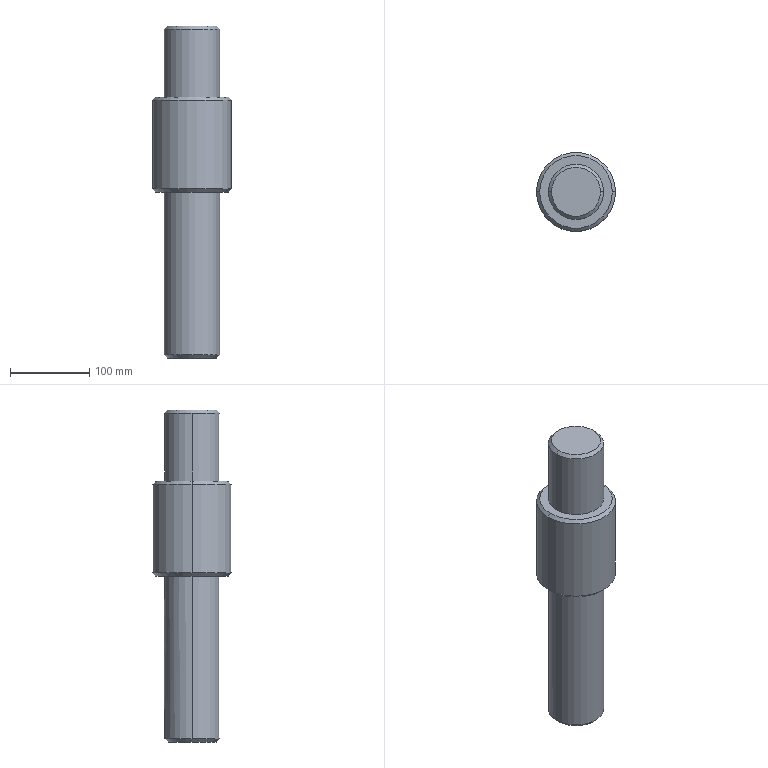Part | SolidWorks | features ICE 2, Chamfer 1, Extrusion 1 | 1 solid | 24 faces | box 100 x 100 x 420 mm | volume 2082883 mm3 | cone 9 | cylinder 8 | plane 7 | commonest cylinder face diameters 70 x4 15 x2 100 x2
STEP:
#1=CARTESIAN_POINT('',(0.,25.,-227.5));
#2=VERTEX_POINT('',#1);
#3=CARTESIAN_POINT('',(7.5,25.,-235.));
#4=VERTEX_POINT('',#3);
#5=CARTESIAN_POINT('',(0.,25.,-235.));
#6=DIRECTION('',(0.,1.,0.));
#7=DIRECTION('',(0.,0.,1.));
#8=AXIS2_PLACEMENT_3D('',#5,#6,#7);
#9=CIRCLE('',#8,7.5);
#10=EDGE_CURVE('',#2,#4,#9,.T.);
#11=ORIENTED_EDGE('',*,*,#10,.F.);
#12=CARTESIAN_POINT('',(0.,35.,-227.5));
#13=VERTEX_POINT('',#12);
#14=CARTESIAN_POINT('',(0.,25.,-227.5));
#15=DIRECTION('',(0.,1.,0.));
#16=VECTOR('',#15,1000.);
#17=LINE('',#14,#16);
#18=EDGE_CURVE('',#2,#13,#17,.T.);
#19=ORIENTED_EDGE('',*,*,#18,.T.);
#20=CARTESIAN_POINT('',(7.5,34.187,-235.));
#21=VERTEX_POINT('',#20);
#22=CARTESIAN_POINT('',(0.,35.,-227.5));
#23=CARTESIAN_POINT('',(0.4904,35.,-227.5));
#24=CARTESIAN_POINT('',(0.9887,34.989,-227.549));
#25=CARTESIAN_POINT('',(1.951,34.949,-227.742));
#26=CARTESIAN_POINT('',(2.419,34.919,-227.884));
#27=CARTESIAN_POINT('',(3.101,34.863,-228.167));
#28=CARTESIAN_POINT('',(3.325,34.842,-228.273));
#29=CARTESIAN_POINT('',(3.758,34.798,-228.505));
#30=CARTESIAN_POINT('',(3.967,34.775,-228.63));
#31=CARTESIAN_POINT('',(4.372,34.726,-228.901));
#32=CARTESIAN_POINT('',(4.568,34.701,-229.047));
#33=CARTESIAN_POINT('',(4.946,34.649,-229.357));
#34=CARTESIAN_POINT('',(5.129,34.623,-229.522));
#35=CARTESIAN_POINT('',(5.651,34.543,-230.044));
#36=CARTESIAN_POINT('',(5.96,34.49,-230.421));
#37=CARTESIAN_POINT('',(6.367,34.416,-231.029));
#38=CARTESIAN_POINT('',(6.493,34.393,-231.238));
#39=CARTESIAN_POINT('',(6.726,34.348,-231.673));
#40=CARTESIAN_POINT('',(6.832,34.327,-231.896));
#41=CARTESIAN_POINT('',(7.114,34.27,-232.575));
#42=CARTESIAN_POINT('',(7.257,34.24,-233.043));
#43=CARTESIAN_POINT('',(7.45,34.198,-234.006));
#44=CARTESIAN_POINT('',(7.5,34.187,-234.503));
#45=CARTESIAN_POINT('',(7.5,34.187,-235.));
#46=B_SPLINE_CURVE_WITH_KNOTS('',3,(#22,#23,#24,#25,#26,#27,#28,#29,#30,#31,#32,#33,#34,#35,#36,#37,#38,#39,#40,#41,#42,#43,#44,#45),.UNSPECIFIED.,.F.,.F.,(4,2,2,2,2,2,2,2,2,2,2,4),(0.01176,0.01323,0.0147,0.01543,0.01617,0.0169,0.01764,0.0191,0.01984,0.02057,0.02204,0.02351),.UNSPECIFIED.);
#47=EDGE_CURVE('',#13,#21,#46,.T.);
#48=ORIENTED_EDGE('',*,*,#47,.T.);
#49=CARTESIAN_POINT('',(7.5,25.,-235.));
#50=DIRECTION('',(0.,1.,0.));
#51=VECTOR('',#50,1000.);
#52=LINE('',#49,#51);
#53=EDGE_CURVE('',#4,#21,#52,.T.);
#54=ORIENTED_EDGE('',*,*,#53,.F.);
#55=EDGE_LOOP('',(#11,#19,#48,#54));
#56=FACE_OUTER_BOUND('',#55,.T.);
#57=CARTESIAN_POINT('',(0.,25.,-235.));
#58=DIRECTION('',(0.,1.,0.));
#59=DIRECTION('',(0.,0.,1.));
#60=AXIS2_PLACEMENT_3D('',#57,#58,#59);
#61=CYLINDRICAL_SURFACE('',#60,7.5);
#62=ADVANCED_FACE('',(#56),#61,.F.);
#63=CARTESIAN_POINT('',(-31.,0.,-270.));
#64=VERTEX_POINT('',#63);
#65=CARTESIAN_POINT('',(-7.5,30.079,-270.));
#66=VERTEX_POINT('',#65);
#67=CARTESIAN_POINT('',(0.,0.,-270.));
#68=DIRECTION('',(0.,0.,-1.));
#69=DIRECTION('',(1.,0.,0.));
#70=AXIS2_PLACEMENT_3D('',#67,#68,#69);
#71=CIRCLE('',#70,31.);
#72=EDGE_CURVE('',#64,#66,#71,.T.);
#73=ORIENTED_EDGE('',*,*,#72,.F.);
#74=CARTESIAN_POINT('',(-35.,0.,-266.));
#75=VERTEX_POINT('',#74);
#76=CARTESIAN_POINT('',(-35.,0.,-266.));
#77=DIRECTION('',(-0.7071,0.,0.7071));
#78=VECTOR('',#77,1000.);
#79=LINE('',#76,#78);
#80=EDGE_CURVE('',#64,#75,#79,.T.);
#81=ORIENTED_EDGE('',*,*,#80,.T.);
#82=CARTESIAN_POINT('',(-7.5,34.187,-266.));
#83=VERTEX_POINT('',#82);
#84=CARTESIAN_POINT('',(0.,0.,-266.));
#85=DIRECTION('',(0.,0.,1.));
#86=DIRECTION('',(1.,0.,0.));
#87=AXIS2_PLACEMENT_3D('',#84,#85,#86);
#88=CIRCLE('',#87,35.);
#89=EDGE_CURVE('',#83,#75,#88,.T.);
#90=ORIENTED_EDGE('',*,*,#89,.F.);
#91=CARTESIAN_POINT('',(-7.5,30.079,-270.));
#92=CARTESIAN_POINT('',(-7.5,31.451,-268.669));
#93=CARTESIAN_POINT('',(-7.5,32.82,-267.335));
#94=CARTESIAN_POINT('',(-7.5,34.187,-266.));
#95=B_SPLINE_CURVE_WITH_KNOTS('',3,(#91,#92,#93,#94),.UNSPECIFIED.,.F.,.F.,(4,4),(0.0194,0.02513),.UNSPECIFIED.);
#96=EDGE_CURVE('',#66,#83,#95,.T.);
#97=ORIENTED_EDGE('',*,*,#96,.F.);
#98=EDGE_LOOP('',(#73,#81,#90,#97));
#99=FACE_OUTER_BOUND('',#98,.T.);
#100=CARTESIAN_POINT('',(0.,0.,-266.));
#101=DIRECTION('',(0.,0.,1.));
#102=DIRECTION('',(1.,0.,0.));
#103=AXIS2_PLACEMENT_3D('',#100,#101,#102);
#104=CONICAL_SURFACE('',#103,35.,0.7854);
#105=ADVANCED_FACE('',(#99),#104,.T.);
#106=ORIENTED_EDGE('',*,*,#80,.F.);
#107=CARTESIAN_POINT('',(31.,0.,-270.));
#108=VERTEX_POINT('',#107);
#109=CARTESIAN_POINT('',(0.,0.,-270.));
#110=DIRECTION('',(0.,0.,-1.));
#111=DIRECTION('',(1.,0.,0.));
#112=AXIS2_PLACEMENT_3D('',#109,#110,#111);
#113=CIRCLE('',#112,31.);
#114=EDGE_CURVE('',#108,#64,#113,.T.);
#115=ORIENTED_EDGE('',*,*,#114,.F.);
#116=CARTESIAN_POINT('',(35.,0.,-266.));
#117=VERTEX_POINT('',#116);
#118=CARTESIAN_POINT('',(35.,0.,-266.));
#119=DIRECTION('',(0.7071,0.,0.7071));
#120=VECTOR('',#119,1000.);
#121=LINE('',#118,#120);
#122=EDGE_CURVE('',#108,#117,#121,.T.);
#123=ORIENTED_EDGE('',*,*,#122,.T.);
#124=CARTESIAN_POINT('',(0.,0.,-266.));
#125=DIRECTION('',(0.,0.,1.));
#126=DIRECTION('',(1.,0.,0.));
#127=AXIS2_PLACEMENT_3D('',#124,#125,#126);
#128=CIRCLE('',#127,35.);
#129=EDGE_CURVE('',#75,#117,#128,.T.);
#130=ORIENTED_EDGE('',*,*,#129,.F.);
#131=EDGE_LOOP('',(#106,#115,#123,#130));
#132=FACE_OUTER_BOUND('',#131,.T.);
#133=CARTESIAN_POINT('',(0.,0.,-266.));
#134=DIRECTION('',(0.,0.,1.));
#135=DIRECTION('',(1.,0.,0.));
#136=AXIS2_PLACEMENT_3D('',#133,#134,#135);
#137=CONICAL_SURFACE('',#136,35.,0.7854);
#138=ADVANCED_FACE('',(#132),#137,.T.);
#139=CARTESIAN_POINT('',(31.,0.,150.));
#140=VERTEX_POINT('',#139);
#141=CARTESIAN_POINT('',(-31.,0.,150.));
#142=VERTEX_POINT('',#141);
#143=CARTESIAN_POINT('',(0.,0.,150.));
#144=DIRECTION('',(0.,0.,1.));
#145=DIRECTION('',(1.,0.,0.));
#146=AXIS2_PLACEMENT_3D('',#143,#144,#145);
#147=CIRCLE('',#146,31.);
#148=EDGE_CURVE('',#140,#142,#147,.T.);
#149=ORIENTED_EDGE('',*,*,#148,.F.);
#150=CARTESIAN_POINT('',(35.,0.,146.));
#151=VERTEX_POINT('',#150);
#152=CARTESIAN_POINT('',(31.,0.,150.));
#153=DIRECTION('',(0.7071,0.,-0.7071));
#154=VECTOR('',#153,1000.);
#155=LINE('',#152,#154);
#156=EDGE_CURVE('',#140,#151,#155,.T.);
#157=ORIENTED_EDGE('',*,*,#156,.T.);
#158=CARTESIAN_POINT('',(-35.,0.,146.));
#159=VERTEX_POINT('',#158);
#160=CARTESIAN_POINT('',(0.,0.,146.));
#161=DIRECTION('',(0.,0.,-1.));
#162=DIRECTION('',(1.,0.,0.));
#163=AXIS2_PLACEMENT_3D('',#160,#161,#162);
#164=CIRCLE('',#163,35.);
#165=EDGE_CURVE('',#159,#151,#164,.T.);
#166=ORIENTED_EDGE('',*,*,#165,.F.);
#167=CARTESIAN_POINT('',(-31.,0.,150.));
#168=DIRECTION('',(-0.7071,0.,-0.7071));
#169=VECTOR('',#168,1000.);
#170=LINE('',#167,#169);
#171=EDGE_CURVE('',#142,#159,#170,.T.);
#172=ORIENTED_EDGE('',*,*,#171,.F.);
#173=EDGE_LOOP('',(#149,#157,#166,#172));
#174=FACE_OUTER_BOUND('',#173,.T.);
#175=CARTESIAN_POINT('',(0.,0.,150.));
#176=DIRECTION('',(0.,0.,-1.));
#177=DIRECTION('',(-1.,0.,0.));
#178=AXIS2_PLACEMENT_3D('',#175,#176,#177);
#179=CONICAL_SURFACE('',#178,31.,0.7854);
#180=ADVANCED_FACE('',(#174),#179,.T.);
#181=CARTESIAN_POINT('',(-46.,0.,-60.));
#182=VERTEX_POINT('',#181);
#183=CARTESIAN_POINT('',(46.,0.,-60.));
#184=VERTEX_POINT('',#183);
#185=CARTESIAN_POINT('',(0.,0.,-60.));
#186=DIRECTION('',(0.,0.,-1.));
#187=DIRECTION('',(1.,0.,0.));
#188=AXIS2_PLACEMENT_3D('',#185,#186,#187);
#189=CIRCLE('',#188,46.);
#190=EDGE_CURVE('',#182,#184,#189,.T.);
#191=ORIENTED_EDGE('',*,*,#190,.F.);
#192=CARTESIAN_POINT('',(-50.,0.,-56.));
#193=VERTEX_POINT('',#192);
#194=CARTESIAN_POINT('',(-50.,0.,-56.));
#195=DIRECTION('',(-0.7071,0.,0.7071));
#196=VECTOR('',#195,1000.);
#197=LINE('',#194,#196);
#198=EDGE_CURVE('',#182,#193,#197,.T.);
#199=ORIENTED_EDGE('',*,*,#198,.T.);
#200=CARTESIAN_POINT('',(50.,0.,-56.));
#201=VERTEX_POINT('',#200);
#202=CARTESIAN_POINT('',(0.,0.,-56.));
#203=DIRECTION('',(0.,0.,1.));
#204=DIRECTION('',(1.,0.,0.));
#205=AXIS2_PLACEMENT_3D('',#202,#203,#204);
#206=CIRCLE('',#205,50.);
#207=EDGE_CURVE('',#201,#193,#206,.T.);
#208=ORIENTED_EDGE('',*,*,#207,.F.);
#209=CARTESIAN_POINT('',(50.,0.,-56.));
#210=DIRECTION('',(0.7071,0.,0.7071));
#211=VECTOR('',#210,1000.);
#212=LINE('',#209,#211);
#213=EDGE_CURVE('',#184,#201,#212,.T.);
#214=ORIENTED_EDGE('',*,*,#213,.F.);
#215=EDGE_LOOP('',(#191,#199,#208,#214));
#216=FACE_OUTER_BOUND('',#215,.T.);
#217=CARTESIAN_POINT('',(0.,0.,-56.));
#218=DIRECTION('',(0.,0.,1.));
#219=DIRECTION('',(1.,0.,0.));
#220=AXIS2_PLACEMENT_3D('',#217,#218,#219);
#221=CONICAL_SURFACE('',#220,50.,0.7854);
#222=ADVANCED_FACE('',(#216),#221,.T.);
#223=CARTESIAN_POINT('',(46.,0.,60.));
#224=VERTEX_POINT('',#223);
#225=CARTESIAN_POINT('',(-46.,0.,60.));
#226=VERTEX_POINT('',#225);
#227=CARTESIAN_POINT('',(0.,0.,60.));
#228=DIRECTION('',(0.,0.,1.));
#229=DIRECTION('',(1.,0.,0.));
#230=AXIS2_PLACEMENT_3D('',#227,#228,#229);
#231=CIRCLE('',#230,46.);
#232=EDGE_CURVE('',#224,#226,#231,.T.);
#233=ORIENTED_EDGE('',*,*,#232,.F.);
#234=CARTESIAN_POINT('',(50.,0.,56.));
#235=VERTEX_POINT('',#234);
#236=CARTESIAN_POINT('',(46.,0.,60.));
#237=DIRECTION('',(0.7071,0.,-0.7071));
#238=VECTOR('',#237,1000.);
#239=LINE('',#236,#238);
#240=EDGE_CURVE('',#224,#235,#239,.T.);
#241=ORIENTED_EDGE('',*,*,#240,.T.);
#242=CARTESIAN_POINT('',(-50.,0.,56.));
#243=VERTEX_POINT('',#242);
#244=CARTESIAN_POINT('',(0.,0.,56.));
#245=DIRECTION('',(0.,0.,-1.));
#246=DIRECTION('',(1.,0.,0.));
#247=AXIS2_PLACEMENT_3D('',#244,#245,#246);
#248=CIRCLE('',#247,50.);
#249=EDGE_CURVE('',#243,#235,#248,.T.);
#250=ORIENTED_EDGE('',*,*,#249,.F.);
#251=CARTESIAN_POINT('',(-46.,0.,60.));
#252=DIRECTION('',(-0.7071,0.,-0.7071));
#253=VECTOR('',#252,1000.);
#254=LINE('',#251,#253);
#255=EDGE_CURVE('',#226,#243,#254,.T.);
#256=ORIENTED_EDGE('',*,*,#255,.F.);
#257=EDGE_LOOP('',(#233,#241,#250,#256));
#258=FACE_OUTER_BOUND('',#257,.T.);
#259=CARTESIAN_POINT('',(0.,0.,60.));
#260=DIRECTION('',(0.,0.,-1.));
#261=DIRECTION('',(-1.,0.,0.));
#262=AXIS2_PLACEMENT_3D('',#259,#260,#261);
#263=CONICAL_SURFACE('',#262,46.,0.7854);
#264=ADVANCED_FACE('',(#258),#263,.T.);
#265=ORIENTED_EDGE('',*,*,#89,.T.);
#266=CARTESIAN_POINT('',(-35.,0.,-60.));
#267=VERTEX_POINT('',#266);
#268=CARTESIAN_POINT('',(-35.,0.,-270.));
#269=DIRECTION('',(0.,0.,1.));
#270=VECTOR('',#269,1000.);
#271=LINE('',#268,#270);
#272=EDGE_CURVE('',#75,#267,#271,.T.);
#273=ORIENTED_EDGE('',*,*,#272,.T.);
#274=CARTESIAN_POINT('',(35.,0.,-60.));
#275=VERTEX_POINT('',#274);
#276=CARTESIAN_POINT('',(0.,0.,-60.));
#277=DIRECTION('',(0.,0.,-1.));
#278=DIRECTION('',(1.,0.,0.));
#279=AXIS2_PLACEMENT_3D('',#276,#277,#278);
#280=CIRCLE('',#279,35.);
#281=EDGE_CURVE('',#267,#275,#280,.T.);
#282=ORIENTED_EDGE('',*,*,#281,.T.);
#283=CARTESIAN_POINT('',(35.,0.,-270.));
#284=DIRECTION('',(0.,0.,1.));
#285=VECTOR('',#284,1000.);
#286=LINE('',#283,#285);
#287=EDGE_CURVE('',#117,#275,#286,.T.);
#288=ORIENTED_EDGE('',*,*,#287,.F.);
#289=CARTESIAN_POINT('',(7.5,34.187,-266.));
#290=VERTEX_POINT('',#289);
#291=CARTESIAN_POINT('',(0.,0.,-266.));
#292=DIRECTION('',(0.,0.,1.));
#293=DIRECTION('',(1.,0.,0.));
#294=AXIS2_PLACEMENT_3D('',#291,#292,#293);
#295=CIRCLE('',#294,35.);
#296=EDGE_CURVE('',#117,#290,#295,.T.);
#297=ORIENTED_EDGE('',*,*,#296,.T.);
#298=CARTESIAN_POINT('',(7.5,34.187,-270.));
#299=DIRECTION('',(0.,0.,-1.));
#300=VECTOR('',#299,1000.);
#301=LINE('',#298,#300);
#302=EDGE_CURVE('',#21,#290,#301,.T.);
#303=ORIENTED_EDGE('',*,*,#302,.F.);
#304=ORIENTED_EDGE('',*,*,#47,.F.);
#305=CARTESIAN_POINT('',(-7.5,34.187,-235.));
#306=VERTEX_POINT('',#305);
#307=CARTESIAN_POINT('',(-7.5,34.187,-235.));
#308=CARTESIAN_POINT('',(-7.5,34.187,-234.503));
#309=CARTESIAN_POINT('',(-7.451,34.198,-234.014));
#310=CARTESIAN_POINT('',(-7.307,34.229,-233.294));
#311=CARTESIAN_POINT('',(-7.248,34.241,-233.055));
#312=CARTESIAN_POINT('',(-7.104,34.271,-232.583));
#313=CARTESIAN_POINT('',(-7.02,34.289,-232.349));
#314=CARTESIAN_POINT('',(-6.737,34.346,-231.668));
#315=CARTESIAN_POINT('',(-6.507,34.391,-231.238));
#316=CARTESIAN_POINT('',(-6.098,34.465,-230.627));
#317=CARTESIAN_POINT('',(-5.951,34.491,-230.429));
#318=CARTESIAN_POINT('',(-5.638,34.543,-230.048));
#319=CARTESIAN_POINT('',(-5.474,34.57,-229.867));
#320=CARTESIAN_POINT('',(-4.956,34.649,-229.35));
#321=CARTESIAN_POINT('',(-4.579,34.702,-229.04));
#322=CARTESIAN_POINT('',(-3.964,34.775,-228.629));
#323=CARTESIAN_POINT('',(-3.752,34.799,-228.501));
#324=CARTESIAN_POINT('',(-3.32,34.843,-228.27));
#325=CARTESIAN_POINT('',(-3.099,34.863,-228.166));
#326=CARTESIAN_POINT('',(-2.648,34.9,-227.979));
#327=CARTESIAN_POINT('',(-2.418,34.917,-227.896));
#328=CARTESIAN_POINT('',(-1.947,34.947,-227.753));
#329=CARTESIAN_POINT('',(-1.706,34.959,-227.692));
#330=CARTESIAN_POINT('',(-0.9787,34.99,-227.548));
#331=CARTESIAN_POINT('',(-0.4909,35.,-227.5));
#332=CARTESIAN_POINT('',(0.,35.,-227.5));
#333=B_SPLINE_CURVE_WITH_KNOTS('',3,(#307,#308,#309,#310,#311,#312,#313,#314,#315,#316,#317,#318,#319,#320,#321,#322,#323,#324,#325,#326,#327,#328,#329,#330,#331,#332),.UNSPECIFIED.,.F.,.F.,(4,2,2,2,2,2,2,2,2,2,2,2,4),(0.,0.00147,0.002205,0.00294,0.00441,0.005146,0.005881,0.007351,0.008086,0.008821,0.009556,0.01029,0.01176),.UNSPECIFIED.);
#334=EDGE_CURVE('',#306,#13,#333,.T.);
#335=ORIENTED_EDGE('',*,*,#334,.F.);
#336=CARTESIAN_POINT('',(-7.5,34.187,-270.));
#337=DIRECTION('',(0.,0.,1.));
#338=VECTOR('',#337,1000.);
#339=LINE('',#336,#338);
#340=EDGE_CURVE('',#83,#306,#339,.T.);
#341=ORIENTED_EDGE('',*,*,#340,.F.);
#342=EDGE_LOOP('',(#265,#273,#282,#288,#297,#303,#304,#335,#341));
#343=FACE_OUTER_BOUND('',#342,.T.);
#344=CARTESIAN_POINT('',(0.,0.,-270.));
#345=DIRECTION('',(0.,0.,1.));
#346=DIRECTION('',(1.,0.,0.));
#347=AXIS2_PLACEMENT_3D('',#344,#345,#346);
#348=CYLINDRICAL_SURFACE('',#347,35.);
#349=ADVANCED_FACE('',(#343),#348,.T.);
#350=ORIENTED_EDGE('',*,*,#249,.T.);
#351=CARTESIAN_POINT('',(50.,0.,60.));
#352=DIRECTION('',(0.,0.,-1.));
#353=VECTOR('',#352,1000.);
#354=LINE('',#351,#353);
#355=EDGE_CURVE('',#235,#201,#354,.T.);
#356=ORIENTED_EDGE('',*,*,#355,.T.);
#357=ORIENTED_EDGE('',*,*,#207,.T.);
#358=CARTESIAN_POINT('',(-50.,0.,60.));
#359=DIRECTION('',(0.,0.,-1.));
#360=VECTOR('',#359,1000.);
#361=LINE('',#358,#360);
#362=EDGE_CURVE('',#243,#193,#361,.T.);
#363=ORIENTED_EDGE('',*,*,#362,.F.);
#364=EDGE_LOOP('',(#350,#356,#357,#363));
#365=FACE_OUTER_BOUND('',#364,.T.);
#366=CARTESIAN_POINT('',(0.,0.,60.));
#367=DIRECTION('',(0.,0.,-1.));
#368=DIRECTION('',(-1.,0.,0.));
#369=AXIS2_PLACEMENT_3D('',#366,#367,#368);
#370=CYLINDRICAL_SURFACE('',#369,50.);
#371=ADVANCED_FACE('',(#365),#370,.T.);
#372=CARTESIAN_POINT('',(-35.,0.,60.));
#373=VERTEX_POINT('',#372);
#374=CARTESIAN_POINT('',(35.,0.,60.));
#375=VERTEX_POINT('',#374);
#376=CARTESIAN_POINT('',(0.,0.,60.));
#377=DIRECTION('',(0.,0.,-1.));
#378=DIRECTION('',(1.,0.,0.));
#379=AXIS2_PLACEMENT_3D('',#376,#377,#378);
#380=CIRCLE('',#379,35.);
#381=EDGE_CURVE('',#373,#375,#380,.T.);
#382=ORIENTED_EDGE('',*,*,#381,.F.);
#383=CARTESIAN_POINT('',(-35.,0.,-270.));
#384=DIRECTION('',(0.,0.,1.));
#385=VECTOR('',#384,1000.);
#386=LINE('',#383,#385);
#387=EDGE_CURVE('',#373,#159,#386,.T.);
#388=ORIENTED_EDGE('',*,*,#387,.T.);
#389=ORIENTED_EDGE('',*,*,#165,.T.);
#390=CARTESIAN_POINT('',(35.,0.,-270.));
#391=DIRECTION('',(0.,0.,1.));
#392=VECTOR('',#391,1000.);
#393=LINE('',#390,#392);
#394=EDGE_CURVE('',#375,#151,#393,.T.);
#395=ORIENTED_EDGE('',*,*,#394,.F.);
#396=EDGE_LOOP('',(#382,#388,#389,#395));
#397=FACE_OUTER_BOUND('',#396,.T.);
#398=CARTESIAN_POINT('',(0.,0.,-270.));
#399=DIRECTION('',(0.,0.,1.));
#400=DIRECTION('',(1.,0.,0.));
#401=AXIS2_PLACEMENT_3D('',#398,#399,#400);
#402=CYLINDRICAL_SURFACE('',#401,35.);
#403=ADVANCED_FACE('',(#397),#402,.T.);
#404=ORIENTED_EDGE('',*,*,#387,.F.);
#405=CARTESIAN_POINT('',(0.,0.,60.));
#406=DIRECTION('',(0.,0.,-1.));
#407=DIRECTION('',(1.,0.,0.));
#408=AXIS2_PLACEMENT_3D('',#405,#406,#407);
#409=CIRCLE('',#408,35.);
#410=EDGE_CURVE('',#375,#373,#409,.T.);
#411=ORIENTED_EDGE('',*,*,#410,.F.);
#412=ORIENTED_EDGE('',*,*,#394,.T.);
#413=CARTESIAN_POINT('',(0.,0.,146.));
#414=DIRECTION('',(0.,0.,-1.));
#415=DIRECTION('',(1.,0.,0.));
#416=AXIS2_PLACEMENT_3D('',#413,#414,#415);
#417=CIRCLE('',#416,35.);
#418=EDGE_CURVE('',#151,#159,#417,.T.);
#419=ORIENTED_EDGE('',*,*,#418,.T.);
#420=EDGE_LOOP('',(#404,#411,#412,#419));
#421=FACE_OUTER_BOUND('',#420,.T.);
#422=CARTESIAN_POINT('',(0.,0.,-270.));
#423=DIRECTION('',(0.,0.,1.));
#424=DIRECTION('',(1.,0.,0.));
#425=AXIS2_PLACEMENT_3D('',#422,#423,#424);
#426=CYLINDRICAL_SURFACE('',#425,35.);
#427=ADVANCED_FACE('',(#421),#426,.T.);
#428=CARTESIAN_POINT('',(0.,0.,150.));
#429=DIRECTION('',(0.,0.,1.));
#430=DIRECTION('',(1.,0.,0.));
#431=AXIS2_PLACEMENT_3D('',#428,#429,#430);
#432=CIRCLE('',#431,31.);
#433=EDGE_CURVE('',#142,#140,#432,.T.);
#434=ORIENTED_EDGE('',*,*,#433,.T.);
#435=ORIENTED_EDGE('',*,*,#148,.T.);
#436=EDGE_LOOP('',(#434,#435));
#437=FACE_OUTER_BOUND('',#436,.T.);
#438=CARTESIAN_POINT('',(0.,0.,150.));
#439=DIRECTION('',(0.,0.,1.));
#440=DIRECTION('',(1.,0.,0.));
#441=AXIS2_PLACEMENT_3D('',#438,#439,#440);
#442=PLANE('',#441);
#443=ADVANCED_FACE('',(#437),#442,.T.);
#444=ORIENTED_EDGE('',*,*,#355,.F.);
#445=CARTESIAN_POINT('',(0.,0.,56.));
#446=DIRECTION('',(0.,0.,-1.));
#447=DIRECTION('',(1.,0.,0.));
#448=AXIS2_PLACEMENT_3D('',#445,#446,#447);
#449=CIRCLE('',#448,50.);
#450=EDGE_CURVE('',#235,#243,#449,.T.);
#451=ORIENTED_EDGE('',*,*,#450,.T.);
#452=ORIENTED_EDGE('',*,*,#362,.T.);
#453=CARTESIAN_POINT('',(0.,0.,-56.));
#454=DIRECTION('',(0.,0.,1.));
#455=DIRECTION('',(1.,0.,0.));
#456=AXIS2_PLACEMENT_3D('',#453,#454,#455);
#457=CIRCLE('',#456,50.);
#458=EDGE_CURVE('',#193,#201,#457,.T.);
#459=ORIENTED_EDGE('',*,*,#458,.T.);
#460=EDGE_LOOP('',(#444,#451,#452,#459));
#461=FACE_OUTER_BOUND('',#460,.T.);
#462=CARTESIAN_POINT('',(0.,0.,60.));
#463=DIRECTION('',(0.,0.,-1.));
#464=DIRECTION('',(-1.,0.,0.));
#465=AXIS2_PLACEMENT_3D('',#462,#463,#464);
#466=CYLINDRICAL_SURFACE('',#465,50.);
#467=ADVANCED_FACE('',(#461),#466,.T.);
#468=CARTESIAN_POINT('',(0.,0.,60.));
#469=DIRECTION('',(0.,0.,1.));
#470=DIRECTION('',(1.,0.,0.));
#471=AXIS2_PLACEMENT_3D('',#468,#469,#470);
#472=CIRCLE('',#471,46.);
#473=EDGE_CURVE('',#226,#224,#472,.T.);
#474=ORIENTED_EDGE('',*,*,#473,.T.);
#475=ORIENTED_EDGE('',*,*,#232,.T.);
#476=EDGE_LOOP('',(#474,#475));
#477=FACE_OUTER_BOUND('',#476,.T.);
#478=ORIENTED_EDGE('',*,*,#410,.T.);
#479=ORIENTED_EDGE('',*,*,#381,.T.);
#480=EDGE_LOOP('',(#478,#479));
#481=FACE_BOUND('',#480,.T.);
#482=CARTESIAN_POINT('',(0.,0.,60.));
#483=DIRECTION('',(0.,0.,1.));
#484=DIRECTION('',(1.,0.,0.));
#485=AXIS2_PLACEMENT_3D('',#482,#483,#484);
#486=PLANE('',#485);
#487=ADVANCED_FACE('',(#477,#481),#486,.T.);
#488=CARTESIAN_POINT('',(0.,0.,-60.));
#489=DIRECTION('',(0.,0.,-1.));
#490=DIRECTION('',(1.,0.,0.));
#491=AXIS2_PLACEMENT_3D('',#488,#489,#490);
#492=CIRCLE('',#491,46.);
#493=EDGE_CURVE('',#184,#182,#492,.T.);
#494=ORIENTED_EDGE('',*,*,#493,.T.);
#495=ORIENTED_EDGE('',*,*,#190,.T.);
#496=EDGE_LOOP('',(#494,#495));
#497=FACE_OUTER_BOUND('',#496,.T.);
#498=CARTESIAN_POINT('',(0.,0.,-60.));
#499=DIRECTION('',(0.,0.,-1.));
#500=DIRECTION('',(1.,0.,0.));
#501=AXIS2_PLACEMENT_3D('',#498,#499,#500);
#502=CIRCLE('',#501,35.);
#503=EDGE_CURVE('',#275,#267,#502,.T.);
#504=ORIENTED_EDGE('',*,*,#503,.F.);
#505=ORIENTED_EDGE('',*,*,#281,.F.);
#506=EDGE_LOOP('',(#504,#505));
#507=FACE_BOUND('',#506,.T.);
#508=CARTESIAN_POINT('',(0.,0.,-60.));
#509=DIRECTION('',(0.,0.,1.));
#510=DIRECTION('',(1.,0.,0.));
#511=AXIS2_PLACEMENT_3D('',#508,#509,#510);
#512=PLANE('',#511);
#513=ADVANCED_FACE('',(#497,#507),#512,.F.);
#514=CARTESIAN_POINT('',(7.5,30.079,-270.));
#515=VERTEX_POINT('',#514);
#516=CARTESIAN_POINT('',(0.,0.,-270.));
#517=DIRECTION('',(0.,0.,-1.));
#518=DIRECTION('',(1.,0.,0.));
#519=AXIS2_PLACEMENT_3D('',#516,#517,#518);
#520=CIRCLE('',#519,31.);
#521=EDGE_CURVE('',#515,#108,#520,.T.);
#522=ORIENTED_EDGE('',*,*,#521,.T.);
#523=ORIENTED_EDGE('',*,*,#114,.T.);
#524=ORIENTED_EDGE('',*,*,#72,.T.);
#525=CARTESIAN_POINT('',(-7.5,25.,-270.));
#526=VERTEX_POINT('',#525);
#527=CARTESIAN_POINT('',(-7.5,0.,-270.));
#528=DIRECTION('',(0.,-1.,0.));
#529=VECTOR('',#528,1000.);
#530=LINE('',#527,#529);
#531=EDGE_CURVE('',#66,#526,#530,.T.);
#532=ORIENTED_EDGE('',*,*,#531,.T.);
#533=CARTESIAN_POINT('',(7.5,25.,-270.));
#534=VERTEX_POINT('',#533);
#535=CARTESIAN_POINT('',(0.,25.,-270.));
#536=DIRECTION('',(-1.,0.,0.));
#537=VECTOR('',#536,1000.);
#538=LINE('',#535,#537);
#539=EDGE_CURVE('',#534,#526,#538,.T.);
#540=ORIENTED_EDGE('',*,*,#539,.F.);
#541=CARTESIAN_POINT('',(7.5,0.,-270.));
#542=DIRECTION('',(0.,1.,0.));
#543=VECTOR('',#542,1000.);
#544=LINE('',#541,#543);
#545=EDGE_CURVE('',#534,#515,#544,.T.);
#546=ORIENTED_EDGE('',*,*,#545,.T.);
#547=EDGE_LOOP('',(#522,#523,#524,#532,#540,#546));
#548=FACE_OUTER_BOUND('',#547,.T.);
#549=CARTESIAN_POINT('',(0.,0.,-270.));
#550=DIRECTION('',(0.,0.,1.));
#551=DIRECTION('',(1.,0.,0.));
#552=AXIS2_PLACEMENT_3D('',#549,#550,#551);
#553=PLANE('',#552);
#554=ADVANCED_FACE('',(#548),#553,.F.);
#555=ORIENTED_EDGE('',*,*,#272,.F.);
#556=ORIENTED_EDGE('',*,*,#129,.T.);
#557=ORIENTED_EDGE('',*,*,#287,.T.);
#558=ORIENTED_EDGE('',*,*,#503,.T.);
#559=EDGE_LOOP('',(#555,#556,#557,#558));
#560=FACE_OUTER_BOUND('',#559,.T.);
#561=CARTESIAN_POINT('',(0.,0.,-270.));
#562=DIRECTION('',(0.,0.,1.));
#563=DIRECTION('',(1.,0.,0.));
#564=AXIS2_PLACEMENT_3D('',#561,#562,#563);
#565=CYLINDRICAL_SURFACE('',#564,35.);
#566=ADVANCED_FACE('',(#560),#565,.T.);
#567=ORIENTED_EDGE('',*,*,#240,.F.);
#568=ORIENTED_EDGE('',*,*,#473,.F.);
#569=ORIENTED_EDGE('',*,*,#255,.T.);
#570=ORIENTED_EDGE('',*,*,#450,.F.);
#571=EDGE_LOOP('',(#567,#568,#569,#570));
#572=FACE_OUTER_BOUND('',#571,.T.);
#573=CARTESIAN_POINT('',(0.,0.,60.));
#574=DIRECTION('',(0.,0.,-1.));
#575=DIRECTION('',(-1.,0.,0.));
#576=AXIS2_PLACEMENT_3D('',#573,#574,#575);
#577=CONICAL_SURFACE('',#576,46.,0.7854);
#578=ADVANCED_FACE('',(#572),#577,.T.);
#579=ORIENTED_EDGE('',*,*,#198,.F.);
#580=ORIENTED_EDGE('',*,*,#493,.F.);
#581=ORIENTED_EDGE('',*,*,#213,.T.);
#582=ORIENTED_EDGE('',*,*,#458,.F.);
#583=EDGE_LOOP('',(#579,#580,#581,#582));
#584=FACE_OUTER_BOUND('',#583,.T.);
#585=CARTESIAN_POINT('',(0.,0.,-56.));
#586=DIRECTION('',(0.,0.,1.));
#587=DIRECTION('',(1.,0.,0.));
#588=AXIS2_PLACEMENT_3D('',#585,#586,#587);
#589=CONICAL_SURFACE('',#588,50.,0.7854);
#590=ADVANCED_FACE('',(#584),#589,.T.);
#591=ORIENTED_EDGE('',*,*,#156,.F.);
#592=ORIENTED_EDGE('',*,*,#433,.F.);
#593=ORIENTED_EDGE('',*,*,#171,.T.);
#594=ORIENTED_EDGE('',*,*,#418,.F.);
#595=EDGE_LOOP('',(#591,#592,#593,#594));
#596=FACE_OUTER_BOUND('',#595,.T.);
#597=CARTESIAN_POINT('',(0.,0.,150.));
#598=DIRECTION('',(0.,0.,-1.));
#599=DIRECTION('',(-1.,0.,0.));
#600=AXIS2_PLACEMENT_3D('',#597,#598,#599);
#601=CONICAL_SURFACE('',#600,31.,0.7854);
#602=ADVANCED_FACE('',(#596),#601,.T.);
#603=ORIENTED_EDGE('',*,*,#122,.F.);
#604=ORIENTED_EDGE('',*,*,#521,.F.);
#605=CARTESIAN_POINT('',(7.5,34.187,-266.));
#606=CARTESIAN_POINT('',(7.5,32.82,-267.335));
#607=CARTESIAN_POINT('',(7.5,31.451,-268.669));
#608=CARTESIAN_POINT('',(7.5,30.079,-270.));
#609=B_SPLINE_CURVE_WITH_KNOTS('',3,(#605,#606,#607,#608),.UNSPECIFIED.,.F.,.F.,(4,4),(0.01813,0.02387),.UNSPECIFIED.);
#610=EDGE_CURVE('',#290,#515,#609,.T.);
#611=ORIENTED_EDGE('',*,*,#610,.F.);
#612=ORIENTED_EDGE('',*,*,#296,.F.);
#613=EDGE_LOOP('',(#603,#604,#611,#612));
#614=FACE_OUTER_BOUND('',#613,.T.);
#615=CARTESIAN_POINT('',(0.,0.,-266.));
#616=DIRECTION('',(0.,0.,1.));
#617=DIRECTION('',(1.,0.,0.));
#618=AXIS2_PLACEMENT_3D('',#615,#616,#617);
#619=CONICAL_SURFACE('',#618,35.,0.7854);
#620=ADVANCED_FACE('',(#614),#619,.T.);
#621=ORIENTED_EDGE('',*,*,#539,.T.);
#622=CARTESIAN_POINT('',(-7.5,25.,-235.));
#623=VERTEX_POINT('',#622);
#624=CARTESIAN_POINT('',(-7.5,25.,-305.));
#625=DIRECTION('',(0.,0.,1.));
#626=VECTOR('',#625,1000.);
#627=LINE('',#624,#626);
#628=EDGE_CURVE('',#526,#623,#627,.T.);
#629=ORIENTED_EDGE('',*,*,#628,.T.);
#630=CARTESIAN_POINT('',(0.,25.,-235.));
#631=DIRECTION('',(0.,1.,0.));
#632=DIRECTION('',(0.,0.,1.));
#633=AXIS2_PLACEMENT_3D('',#630,#631,#632);
#634=CIRCLE('',#633,7.5);
#635=EDGE_CURVE('',#623,#2,#634,.T.);
#636=ORIENTED_EDGE('',*,*,#635,.T.);
#637=ORIENTED_EDGE('',*,*,#10,.T.);
#638=CARTESIAN_POINT('',(7.5,25.,-305.));
#639=DIRECTION('',(0.,0.,-1.));
#640=VECTOR('',#639,1000.);
#641=LINE('',#638,#640);
#642=EDGE_CURVE('',#4,#534,#641,.T.);
#643=ORIENTED_EDGE('',*,*,#642,.T.);
#644=EDGE_LOOP('',(#621,#629,#636,#637,#643));
#645=FACE_OUTER_BOUND('',#644,.T.);
#646=CARTESIAN_POINT('',(0.,25.,-235.));
#647=DIRECTION('',(0.,1.,0.));
#648=DIRECTION('',(0.,0.,1.));
#649=AXIS2_PLACEMENT_3D('',#646,#647,#648);
#650=PLANE('',#649);
#651=ADVANCED_FACE('',(#645),#650,.T.);
#652=ORIENTED_EDGE('',*,*,#96,.T.);
#653=ORIENTED_EDGE('',*,*,#340,.T.);
#654=CARTESIAN_POINT('',(-7.5,25.,-235.));
#655=DIRECTION('',(0.,1.,0.));
#656=VECTOR('',#655,1000.);
#657=LINE('',#654,#656);
#658=EDGE_CURVE('',#623,#306,#657,.T.);
#659=ORIENTED_EDGE('',*,*,#658,.F.);
#660=ORIENTED_EDGE('',*,*,#628,.F.);
#661=ORIENTED_EDGE('',*,*,#531,.F.);
#662=EDGE_LOOP('',(#652,#653,#659,#660,#661));
#663=FACE_OUTER_BOUND('',#662,.T.);
#664=CARTESIAN_POINT('',(-7.5,25.,-305.));
#665=DIRECTION('',(-1.,0.,0.));
#666=DIRECTION('',(0.,0.,1.));
#667=AXIS2_PLACEMENT_3D('',#664,#665,#666);
#668=PLANE('',#667);
#669=ADVANCED_FACE('',(#663),#668,.F.);
#670=ORIENTED_EDGE('',*,*,#642,.F.);
#671=ORIENTED_EDGE('',*,*,#53,.T.);
#672=ORIENTED_EDGE('',*,*,#302,.T.);
#673=ORIENTED_EDGE('',*,*,#610,.T.);
#674=ORIENTED_EDGE('',*,*,#545,.F.);
#675=EDGE_LOOP('',(#670,#671,#672,#673,#674));
#676=FACE_OUTER_BOUND('',#675,.T.);
#677=CARTESIAN_POINT('',(7.5,25.,-305.));
#678=DIRECTION('',(1.,0.,0.));
#679=DIRECTION('',(0.,0.,-1.));
#680=AXIS2_PLACEMENT_3D('',#677,#678,#679);
#681=PLANE('',#680);
#682=ADVANCED_FACE('',(#676),#681,.F.);
#683=ORIENTED_EDGE('',*,*,#18,.F.);
#684=ORIENTED_EDGE('',*,*,#635,.F.);
#685=ORIENTED_EDGE('',*,*,#658,.T.);
#686=ORIENTED_EDGE('',*,*,#334,.T.);
#687=EDGE_LOOP('',(#683,#684,#685,#686));
#688=FACE_OUTER_BOUND('',#687,.T.);
#689=CARTESIAN_POINT('',(0.,25.,-235.));
#690=DIRECTION('',(0.,1.,0.));
#691=DIRECTION('',(0.,0.,1.));
#692=AXIS2_PLACEMENT_3D('',#689,#690,#691);
#693=CYLINDRICAL_SURFACE('',#692,7.5);
#694=ADVANCED_FACE('',(#688),#693,.F.);
#695=CLOSED_SHELL('',(#62,#105,#138,#180,#222,#264,#349,#371,#403,#427,#443,#467,#487,#513,#554,#566,#578,#590,#602,#620,#651,#669,#682,#694));
#696=MANIFOLD_SOLID_BREP('',#695);
#697=CARTESIAN_POINT('',(0.,0.,0.));
#698=DIRECTION('',(0.,0.,1.));
#699=DIRECTION('',(1.,0.,0.));
#700=AXIS2_PLACEMENT_3D('',#697,#698,#699);
#701=(LENGTH_UNIT()NAMED_UNIT(*)SI_UNIT(.MILLI.,.METRE.));
#702=UNCERTAINTY_MEASURE_WITH_UNIT(LENGTH_MEASURE(0.00001),#701,'','');
#703=(NAMED_UNIT(*)PLANE_ANGLE_UNIT()SI_UNIT($,.RADIAN.));
#704=(NAMED_UNIT(*)SI_UNIT($,.STERADIAN.)SOLID_ANGLE_UNIT());
#705=(GEOMETRIC_REPRESENTATION_CONTEXT(3)GLOBAL_UNCERTAINTY_ASSIGNED_CONTEXT((#702))GLOBAL_UNIT_ASSIGNED_CONTEXT((#701,#703,#704))REPRESENTATION_CONTEXT('',''));
#706=ADVANCED_BREP_SHAPE_REPRESENTATION('',(#696,#700),#705);